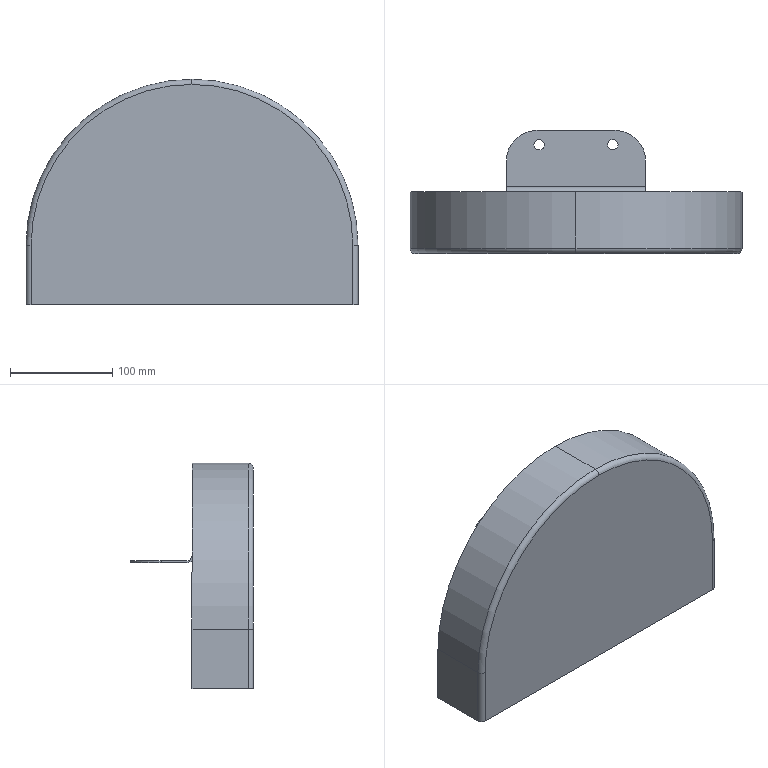Part | NX | features BREP 1 | 1 solid | 40 faces | box 324 x 120 x 220 mm | volume 283297 mm3 | cylinder 18 | plane 18 | torus 4 | commonest cylinder face diameters 10 x9 6 x2 60 x2 320 x2 324 x2 14 x1
STEP:
#1=CARTESIAN_POINT('',(193.612,71.603,383.));
#2=VERTEX_POINT('',#1);
#3=CARTESIAN_POINT('',(193.612,71.603,385.));
#4=VERTEX_POINT('',#3);
#5=CARTESIAN_POINT('',(193.612,71.603,326.345));
#6=DIRECTION('',(0.,0.,-1.));
#7=VECTOR('',#6,1000.);
#8=LINE('',#5,#7);
#9=EDGE_CURVE('',#2,#4,#8,.F.);
#10=ORIENTED_EDGE('',*,*,#9,.T.);
#11=CARTESIAN_POINT('',(202.388,76.397,385.));
#12=VERTEX_POINT('',#11);
#13=CARTESIAN_POINT('',(198.,74.,385.));
#14=DIRECTION('',(0.,0.,-1.));
#15=DIRECTION('',(1.,0.,0.));
#16=AXIS2_PLACEMENT_3D('',#13,#14,#15);
#17=CIRCLE('',#16,5.);
#18=EDGE_CURVE('',#12,#4,#17,.T.);
#19=ORIENTED_EDGE('',*,*,#18,.F.);
#20=CARTESIAN_POINT('',(202.388,76.397,383.));
#21=VERTEX_POINT('',#20);
#22=CARTESIAN_POINT('',(202.388,76.397,326.345));
#23=DIRECTION('',(0.,0.,-1.));
#24=VECTOR('',#23,1000.);
#25=LINE('',#22,#24);
#26=EDGE_CURVE('',#21,#12,#25,.F.);
#27=ORIENTED_EDGE('',*,*,#26,.F.);
#28=CARTESIAN_POINT('',(198.,74.,383.));
#29=DIRECTION('',(0.,0.,-1.));
#30=DIRECTION('',(1.,0.,0.));
#31=AXIS2_PLACEMENT_3D('',#28,#29,#30);
#32=CIRCLE('',#31,5.);
#33=EDGE_CURVE('',#21,#2,#32,.T.);
#34=ORIENTED_EDGE('',*,*,#33,.T.);
#35=EDGE_LOOP('',(#10,#19,#27,#34));
#36=FACE_BOUND('',#35,.T.);
#37=CARTESIAN_POINT('',(198.,74.,383.1));
#38=DIRECTION('',(0.,0.,1.));
#39=DIRECTION('',(-0.8776,-0.4794,0.));
#40=AXIS2_PLACEMENT_3D('',#37,#38,#39);
#41=CYLINDRICAL_SURFACE('',#40,5.);
#42=ADVANCED_FACE('',(#36),#41,.F.);
#43=ORIENTED_EDGE('',*,*,#26,.T.);
#44=CARTESIAN_POINT('',(198.,74.,385.));
#45=DIRECTION('',(0.,0.,-1.));
#46=DIRECTION('',(1.,0.,0.));
#47=AXIS2_PLACEMENT_3D('',#44,#45,#46);
#48=CIRCLE('',#47,5.);
#49=EDGE_CURVE('',#4,#12,#48,.T.);
#50=ORIENTED_EDGE('',*,*,#49,.F.);
#51=ORIENTED_EDGE('',*,*,#9,.F.);
#52=CARTESIAN_POINT('',(198.,74.,383.));
#53=DIRECTION('',(0.,0.,-1.));
#54=DIRECTION('',(1.,0.,0.));
#55=AXIS2_PLACEMENT_3D('',#52,#53,#54);
#56=CIRCLE('',#55,5.);
#57=EDGE_CURVE('',#2,#21,#56,.T.);
#58=ORIENTED_EDGE('',*,*,#57,.T.);
#59=EDGE_LOOP('',(#43,#50,#51,#58));
#60=FACE_BOUND('',#59,.T.);
#61=CARTESIAN_POINT('',(198.,74.,383.1));
#62=DIRECTION('',(0.,0.,1.));
#63=DIRECTION('',(-0.8776,-0.4794,0.));
#64=AXIS2_PLACEMENT_3D('',#61,#62,#63);
#65=CYLINDRICAL_SURFACE('',#64,5.);
#66=ADVANCED_FACE('',(#60),#65,.F.);
#67=CARTESIAN_POINT('',(240.,26.,393.));
#68=VERTEX_POINT('',#67);
#69=CARTESIAN_POINT('',(230.,26.,393.));
#70=VERTEX_POINT('',#69);
#71=CARTESIAN_POINT('',(235.,26.,393.));
#72=DIRECTION('',(-1.,0.,0.));
#73=VECTOR('',#72,1000.);
#74=LINE('',#71,#73);
#75=EDGE_CURVE('',#68,#70,#74,.T.);
#76=ORIENTED_EDGE('',*,*,#75,.T.);
#77=CARTESIAN_POINT('',(230.,28.,393.));
#78=VERTEX_POINT('',#77);
#79=CARTESIAN_POINT('',(230.,27.,393.));
#80=DIRECTION('',(0.,-1.,0.));
#81=VECTOR('',#80,1000.);
#82=LINE('',#79,#81);
#83=EDGE_CURVE('',#78,#70,#82,.T.);
#84=ORIENTED_EDGE('',*,*,#83,.F.);
#85=CARTESIAN_POINT('',(240.,28.,393.));
#86=VERTEX_POINT('',#85);
#87=CARTESIAN_POINT('',(235.,28.,393.));
#88=DIRECTION('',(1.,0.,0.));
#89=VECTOR('',#88,1000.);
#90=LINE('',#87,#89);
#91=EDGE_CURVE('',#78,#86,#90,.T.);
#92=ORIENTED_EDGE('',*,*,#91,.T.);
#93=CARTESIAN_POINT('',(240.,27.,393.));
#94=DIRECTION('',(0.,-1.,0.));
#95=VECTOR('',#94,1000.);
#96=LINE('',#93,#95);
#97=EDGE_CURVE('',#86,#68,#96,.T.);
#98=ORIENTED_EDGE('',*,*,#97,.T.);
#99=EDGE_LOOP('',(#76,#84,#92,#98));
#100=FACE_BOUND('',#99,.T.);
#101=CARTESIAN_POINT('',(94.,28.,393.));
#102=DIRECTION('',(0.,0.,1.));
#103=DIRECTION('',(1.,0.,0.));
#104=AXIS2_PLACEMENT_3D('',#101,#102,#103);
#105=PLANE('',#104);
#106=ADVANCED_FACE('',(#100),#105,.F.);
#107=CARTESIAN_POINT('',(94.,33.,385.));
#108=VERTEX_POINT('',#107);
#109=CARTESIAN_POINT('',(230.,33.,385.));
#110=VERTEX_POINT('',#109);
#111=CARTESIAN_POINT('',(162.,33.,385.));
#112=DIRECTION('',(1.,0.,0.));
#113=VECTOR('',#112,1000.);
#114=LINE('',#111,#113);
#115=EDGE_CURVE('',#108,#110,#114,.T.);
#116=ORIENTED_EDGE('',*,*,#115,.F.);
#117=CARTESIAN_POINT('',(94.,28.,390.));
#118=VERTEX_POINT('',#117);
#119=CARTESIAN_POINT('',(94.,33.,390.));
#120=DIRECTION('',(1.,0.,0.));
#121=DIRECTION('',(0.,0.,-1.));
#122=AXIS2_PLACEMENT_3D('',#119,#120,#121);
#123=CIRCLE('',#122,5.);
#124=EDGE_CURVE('',#118,#108,#123,.T.);
#125=ORIENTED_EDGE('',*,*,#124,.F.);
#126=CARTESIAN_POINT('',(230.,28.,390.));
#127=VERTEX_POINT('',#126);
#128=CARTESIAN_POINT('',(162.,28.,390.));
#129=DIRECTION('',(1.,0.,0.));
#130=VECTOR('',#129,1000.);
#131=LINE('',#128,#130);
#132=EDGE_CURVE('',#118,#127,#131,.T.);
#133=ORIENTED_EDGE('',*,*,#132,.T.);
#134=CARTESIAN_POINT('',(230.,33.,390.));
#135=DIRECTION('',(-1.,0.,0.));
#136=DIRECTION('',(0.,0.,-1.));
#137=AXIS2_PLACEMENT_3D('',#134,#135,#136);
#138=CIRCLE('',#137,5.);
#139=EDGE_CURVE('',#110,#127,#138,.T.);
#140=ORIENTED_EDGE('',*,*,#139,.F.);
#141=EDGE_LOOP('',(#116,#125,#133,#140));
#142=FACE_BOUND('',#141,.T.);
#143=CARTESIAN_POINT('',(162.,33.,390.));
#144=DIRECTION('',(1.,0.,0.));
#145=DIRECTION('',(0.,1.,0.));
#146=AXIS2_PLACEMENT_3D('',#143,#144,#145);
#147=CYLINDRICAL_SURFACE('',#146,5.);
#148=ADVANCED_FACE('',(#142),#147,.F.);
#149=CARTESIAN_POINT('',(94.,26.,393.));
#150=VERTEX_POINT('',#149);
#151=CARTESIAN_POINT('',(84.,26.,393.));
#152=VERTEX_POINT('',#151);
#153=CARTESIAN_POINT('',(89.,26.,393.));
#154=DIRECTION('',(-1.,0.,0.));
#155=VECTOR('',#154,1000.);
#156=LINE('',#153,#155);
#157=EDGE_CURVE('',#150,#152,#156,.T.);
#158=ORIENTED_EDGE('',*,*,#157,.T.);
#159=CARTESIAN_POINT('',(84.,28.,393.));
#160=VERTEX_POINT('',#159);
#161=CARTESIAN_POINT('',(84.,27.,393.));
#162=DIRECTION('',(0.,-1.,0.));
#163=VECTOR('',#162,1000.);
#164=LINE('',#161,#163);
#165=EDGE_CURVE('',#160,#152,#164,.T.);
#166=ORIENTED_EDGE('',*,*,#165,.F.);
#167=CARTESIAN_POINT('',(94.,28.,393.));
#168=VERTEX_POINT('',#167);
#169=CARTESIAN_POINT('',(89.,28.,393.));
#170=DIRECTION('',(1.,0.,0.));
#171=VECTOR('',#170,1000.);
#172=LINE('',#169,#171);
#173=EDGE_CURVE('',#160,#168,#172,.T.);
#174=ORIENTED_EDGE('',*,*,#173,.T.);
#175=CARTESIAN_POINT('',(94.,27.,393.));
#176=DIRECTION('',(0.,-1.,0.));
#177=VECTOR('',#176,1000.);
#178=LINE('',#175,#177);
#179=EDGE_CURVE('',#168,#150,#178,.T.);
#180=ORIENTED_EDGE('',*,*,#179,.T.);
#181=EDGE_LOOP('',(#158,#166,#174,#180));
#182=FACE_BOUND('',#181,.T.);
#183=CARTESIAN_POINT('',(94.,28.,393.));
#184=DIRECTION('',(0.,0.,1.));
#185=DIRECTION('',(1.,0.,0.));
#186=AXIS2_PLACEMENT_3D('',#183,#184,#185);
#187=PLANE('',#186);
#188=ADVANCED_FACE('',(#182),#187,.F.);
#189=CARTESIAN_POINT('',(230.,33.,383.));
#190=VERTEX_POINT('',#189);
#191=CARTESIAN_POINT('',(230.,26.,390.));
#192=VERTEX_POINT('',#191);
#193=CARTESIAN_POINT('',(230.,33.,390.));
#194=DIRECTION('',(-1.,0.,0.));
#195=DIRECTION('',(0.,0.,-1.));
#196=AXIS2_PLACEMENT_3D('',#193,#194,#195);
#197=CIRCLE('',#196,7.);
#198=EDGE_CURVE('',#190,#192,#197,.T.);
#199=ORIENTED_EDGE('',*,*,#198,.T.);
#200=CARTESIAN_POINT('',(94.,26.,390.));
#201=VERTEX_POINT('',#200);
#202=CARTESIAN_POINT('',(162.,26.,390.));
#203=DIRECTION('',(1.,0.,0.));
#204=VECTOR('',#203,1000.);
#205=LINE('',#202,#204);
#206=EDGE_CURVE('',#201,#192,#205,.T.);
#207=ORIENTED_EDGE('',*,*,#206,.F.);
#208=CARTESIAN_POINT('',(94.,33.,383.));
#209=VERTEX_POINT('',#208);
#210=CARTESIAN_POINT('',(94.,33.,390.));
#211=DIRECTION('',(1.,0.,0.));
#212=DIRECTION('',(0.,0.,-1.));
#213=AXIS2_PLACEMENT_3D('',#210,#211,#212);
#214=CIRCLE('',#213,7.);
#215=EDGE_CURVE('',#201,#209,#214,.T.);
#216=ORIENTED_EDGE('',*,*,#215,.T.);
#217=CARTESIAN_POINT('',(162.,33.,383.));
#218=DIRECTION('',(1.,0.,0.));
#219=VECTOR('',#218,1000.);
#220=LINE('',#217,#219);
#221=EDGE_CURVE('',#209,#190,#220,.T.);
#222=ORIENTED_EDGE('',*,*,#221,.T.);
#223=EDGE_LOOP('',(#199,#207,#216,#222));
#224=FACE_BOUND('',#223,.T.);
#225=CARTESIAN_POINT('',(162.,33.,390.));
#226=DIRECTION('',(1.,0.,0.));
#227=DIRECTION('',(0.,1.,0.));
#228=AXIS2_PLACEMENT_3D('',#225,#226,#227);
#229=CYLINDRICAL_SURFACE('',#228,7.);
#230=ADVANCED_FACE('',(#224),#229,.T.);
#231=CARTESIAN_POINT('',(121.612,71.603,383.));
#232=VERTEX_POINT('',#231);
#233=CARTESIAN_POINT('',(121.612,71.603,385.));
#234=VERTEX_POINT('',#233);
#235=CARTESIAN_POINT('',(121.612,71.603,326.345));
#236=DIRECTION('',(0.,0.,-1.));
#237=VECTOR('',#236,1000.);
#238=LINE('',#235,#237);
#239=EDGE_CURVE('',#232,#234,#238,.F.);
#240=ORIENTED_EDGE('',*,*,#239,.T.);
#241=CARTESIAN_POINT('',(130.388,76.397,385.));
#242=VERTEX_POINT('',#241);
#243=CARTESIAN_POINT('',(126.,74.,385.));
#244=DIRECTION('',(0.,0.,-1.));
#245=DIRECTION('',(1.,0.,0.));
#246=AXIS2_PLACEMENT_3D('',#243,#244,#245);
#247=CIRCLE('',#246,5.);
#248=EDGE_CURVE('',#242,#234,#247,.T.);
#249=ORIENTED_EDGE('',*,*,#248,.F.);
#250=CARTESIAN_POINT('',(130.388,76.397,383.));
#251=VERTEX_POINT('',#250);
#252=CARTESIAN_POINT('',(130.388,76.397,326.345));
#253=DIRECTION('',(0.,0.,-1.));
#254=VECTOR('',#253,1000.);
#255=LINE('',#252,#254);
#256=EDGE_CURVE('',#251,#242,#255,.F.);
#257=ORIENTED_EDGE('',*,*,#256,.F.);
#258=CARTESIAN_POINT('',(126.,74.,383.));
#259=DIRECTION('',(0.,0.,-1.));
#260=DIRECTION('',(1.,0.,0.));
#261=AXIS2_PLACEMENT_3D('',#258,#259,#260);
#262=CIRCLE('',#261,5.);
#263=EDGE_CURVE('',#251,#232,#262,.T.);
#264=ORIENTED_EDGE('',*,*,#263,.T.);
#265=EDGE_LOOP('',(#240,#249,#257,#264));
#266=FACE_BOUND('',#265,.T.);
#267=CARTESIAN_POINT('',(126.,74.,383.1));
#268=DIRECTION('',(0.,0.,1.));
#269=DIRECTION('',(-0.8776,-0.4794,0.));
#270=AXIS2_PLACEMENT_3D('',#267,#268,#269);
#271=CYLINDRICAL_SURFACE('',#270,5.);
#272=ADVANCED_FACE('',(#266),#271,.F.);
#273=ORIENTED_EDGE('',*,*,#256,.T.);
#274=CARTESIAN_POINT('',(126.,74.,385.));
#275=DIRECTION('',(0.,0.,-1.));
#276=DIRECTION('',(1.,0.,0.));
#277=AXIS2_PLACEMENT_3D('',#274,#275,#276);
#278=CIRCLE('',#277,5.);
#279=EDGE_CURVE('',#234,#242,#278,.T.);
#280=ORIENTED_EDGE('',*,*,#279,.F.);
#281=ORIENTED_EDGE('',*,*,#239,.F.);
#282=CARTESIAN_POINT('',(126.,74.,383.));
#283=DIRECTION('',(0.,0.,-1.));
#284=DIRECTION('',(1.,0.,0.));
#285=AXIS2_PLACEMENT_3D('',#282,#283,#284);
#286=CIRCLE('',#285,5.);
#287=EDGE_CURVE('',#232,#251,#286,.T.);
#288=ORIENTED_EDGE('',*,*,#287,.T.);
#289=EDGE_LOOP('',(#273,#280,#281,#288));
#290=FACE_BOUND('',#289,.T.);
#291=CARTESIAN_POINT('',(126.,74.,383.1));
#292=DIRECTION('',(0.,0.,1.));
#293=DIRECTION('',(-0.8776,-0.4794,0.));
#294=AXIS2_PLACEMENT_3D('',#291,#292,#293);
#295=CYLINDRICAL_SURFACE('',#294,5.);
#296=ADVANCED_FACE('',(#290),#295,.F.);
#297=CARTESIAN_POINT('',(94.,58.,383.));
#298=VERTEX_POINT('',#297);
#299=CARTESIAN_POINT('',(94.,58.,385.));
#300=VERTEX_POINT('',#299);
#301=CARTESIAN_POINT('',(94.,58.,384.));
#302=DIRECTION('',(0.,0.,1.));
#303=VECTOR('',#302,1000.);
#304=LINE('',#301,#303);
#305=EDGE_CURVE('',#298,#300,#304,.T.);
#306=ORIENTED_EDGE('',*,*,#305,.F.);
#307=CARTESIAN_POINT('',(94.,45.5,383.));
#308=DIRECTION('',(0.,-1.,0.));
#309=VECTOR('',#308,1000.);
#310=LINE('',#307,#309);
#311=EDGE_CURVE('',#298,#209,#310,.T.);
#312=ORIENTED_EDGE('',*,*,#311,.T.);
#313=ORIENTED_EDGE('',*,*,#215,.F.);
#314=CARTESIAN_POINT('',(94.,26.,391.5));
#315=DIRECTION('',(0.,0.,-1.));
#316=VECTOR('',#315,1000.);
#317=LINE('',#314,#316);
#318=EDGE_CURVE('',#150,#201,#317,.T.);
#319=ORIENTED_EDGE('',*,*,#318,.F.);
#320=ORIENTED_EDGE('',*,*,#179,.F.);
#321=CARTESIAN_POINT('',(94.,28.,391.5));
#322=DIRECTION('',(0.,0.,-1.));
#323=VECTOR('',#322,1000.);
#324=LINE('',#321,#323);
#325=EDGE_CURVE('',#168,#118,#324,.T.);
#326=ORIENTED_EDGE('',*,*,#325,.T.);
#327=ORIENTED_EDGE('',*,*,#124,.T.);
#328=CARTESIAN_POINT('',(94.,45.5,385.));
#329=DIRECTION('',(0.,1.,0.));
#330=VECTOR('',#329,1000.);
#331=LINE('',#328,#330);
#332=EDGE_CURVE('',#108,#300,#331,.T.);
#333=ORIENTED_EDGE('',*,*,#332,.T.);
#334=EDGE_LOOP('',(#306,#312,#313,#319,#320,#326,#327,#333));
#335=FACE_BOUND('',#334,.T.);
#336=CARTESIAN_POINT('',(94.,28.,383.));
#337=DIRECTION('',(1.,0.,0.));
#338=DIRECTION('',(0.,-1.,0.));
#339=AXIS2_PLACEMENT_3D('',#336,#337,#338);
#340=PLANE('',#339);
#341=ADVANCED_FACE('',(#335),#340,.F.);
#342=CARTESIAN_POINT('',(124.,88.,385.));
#343=VERTEX_POINT('',#342);
#344=CARTESIAN_POINT('',(124.,58.,385.));
#345=DIRECTION('',(0.,0.,-1.));
#346=DIRECTION('',(1.,0.,0.));
#347=AXIS2_PLACEMENT_3D('',#344,#345,#346);
#348=CIRCLE('',#347,30.);
#349=EDGE_CURVE('',#300,#343,#348,.T.);
#350=ORIENTED_EDGE('',*,*,#349,.T.);
#351=CARTESIAN_POINT('',(124.,88.,383.));
#352=VERTEX_POINT('',#351);
#353=CARTESIAN_POINT('',(124.,88.,388.));
#354=DIRECTION('',(0.,0.,1.));
#355=VECTOR('',#354,1000.);
#356=LINE('',#353,#355);
#357=EDGE_CURVE('',#352,#343,#356,.T.);
#358=ORIENTED_EDGE('',*,*,#357,.F.);
#359=CARTESIAN_POINT('',(124.,58.,383.));
#360=DIRECTION('',(0.,0.,1.));
#361=DIRECTION('',(1.,0.,0.));
#362=AXIS2_PLACEMENT_3D('',#359,#360,#361);
#363=CIRCLE('',#362,30.);
#364=EDGE_CURVE('',#352,#298,#363,.T.);
#365=ORIENTED_EDGE('',*,*,#364,.T.);
#366=ORIENTED_EDGE('',*,*,#305,.T.);
#367=EDGE_LOOP('',(#350,#358,#365,#366));
#368=FACE_BOUND('',#367,.T.);
#369=CARTESIAN_POINT('',(124.,58.,388.));
#370=DIRECTION('',(0.,0.,1.));
#371=DIRECTION('',(0.,-1.,0.));
#372=AXIS2_PLACEMENT_3D('',#369,#370,#371);
#373=CYLINDRICAL_SURFACE('',#372,30.);
#374=ADVANCED_FACE('',(#368),#373,.T.);
#375=CARTESIAN_POINT('',(230.,58.,383.));
#376=VERTEX_POINT('',#375);
#377=CARTESIAN_POINT('',(230.,58.,385.));
#378=VERTEX_POINT('',#377);
#379=CARTESIAN_POINT('',(230.,58.,384.));
#380=DIRECTION('',(0.,0.,1.));
#381=VECTOR('',#380,1000.);
#382=LINE('',#379,#381);
#383=EDGE_CURVE('',#376,#378,#382,.T.);
#384=ORIENTED_EDGE('',*,*,#383,.T.);
#385=CARTESIAN_POINT('',(230.,45.5,385.));
#386=DIRECTION('',(0.,-1.,0.));
#387=VECTOR('',#386,1000.);
#388=LINE('',#385,#387);
#389=EDGE_CURVE('',#378,#110,#388,.T.);
#390=ORIENTED_EDGE('',*,*,#389,.T.);
#391=ORIENTED_EDGE('',*,*,#139,.T.);
#392=CARTESIAN_POINT('',(230.,28.,391.5));
#393=DIRECTION('',(0.,0.,1.));
#394=VECTOR('',#393,1000.);
#395=LINE('',#392,#394);
#396=EDGE_CURVE('',#127,#78,#395,.T.);
#397=ORIENTED_EDGE('',*,*,#396,.T.);
#398=ORIENTED_EDGE('',*,*,#83,.T.);
#399=CARTESIAN_POINT('',(230.,26.,391.5));
#400=DIRECTION('',(0.,0.,-1.));
#401=VECTOR('',#400,1000.);
#402=LINE('',#399,#401);
#403=EDGE_CURVE('',#70,#192,#402,.T.);
#404=ORIENTED_EDGE('',*,*,#403,.T.);
#405=ORIENTED_EDGE('',*,*,#198,.F.);
#406=CARTESIAN_POINT('',(230.,45.5,383.));
#407=DIRECTION('',(0.,-1.,0.));
#408=VECTOR('',#407,1000.);
#409=LINE('',#406,#408);
#410=EDGE_CURVE('',#376,#190,#409,.T.);
#411=ORIENTED_EDGE('',*,*,#410,.F.);
#412=EDGE_LOOP('',(#384,#390,#391,#397,#398,#404,#405,#411));
#413=FACE_BOUND('',#412,.T.);
#414=CARTESIAN_POINT('',(230.,88.,383.));
#415=DIRECTION('',(-1.,0.,0.));
#416=DIRECTION('',(0.,1.,0.));
#417=AXIS2_PLACEMENT_3D('',#414,#415,#416);
#418=PLANE('',#417);
#419=ADVANCED_FACE('',(#413),#418,.F.);
#420=CARTESIAN_POINT('',(200.,88.,383.));
#421=VERTEX_POINT('',#420);
#422=CARTESIAN_POINT('',(162.,88.,383.));
#423=DIRECTION('',(1.,0.,0.));
#424=VECTOR('',#423,1000.);
#425=LINE('',#422,#424);
#426=EDGE_CURVE('',#352,#421,#425,.T.);
#427=ORIENTED_EDGE('',*,*,#426,.F.);
#428=ORIENTED_EDGE('',*,*,#357,.T.);
#429=CARTESIAN_POINT('',(200.,88.,385.));
#430=VERTEX_POINT('',#429);
#431=CARTESIAN_POINT('',(162.,88.,385.));
#432=DIRECTION('',(1.,0.,0.));
#433=VECTOR('',#432,1000.);
#434=LINE('',#431,#433);
#435=EDGE_CURVE('',#343,#430,#434,.T.);
#436=ORIENTED_EDGE('',*,*,#435,.T.);
#437=CARTESIAN_POINT('',(200.,88.,384.));
#438=DIRECTION('',(0.,0.,1.));
#439=VECTOR('',#438,1000.);
#440=LINE('',#437,#439);
#441=EDGE_CURVE('',#421,#430,#440,.T.);
#442=ORIENTED_EDGE('',*,*,#441,.F.);
#443=EDGE_LOOP('',(#427,#428,#436,#442));
#444=FACE_BOUND('',#443,.T.);
#445=CARTESIAN_POINT('',(230.,88.,383.));
#446=DIRECTION('',(0.,1.,0.));
#447=DIRECTION('',(1.,0.,0.));
#448=AXIS2_PLACEMENT_3D('',#445,#446,#447);
#449=PLANE('',#448);
#450=ADVANCED_FACE('',(#444),#449,.T.);
#451=CARTESIAN_POINT('',(200.,58.,385.));
#452=DIRECTION('',(0.,0.,-1.));
#453=DIRECTION('',(-1.,0.,0.));
#454=AXIS2_PLACEMENT_3D('',#451,#452,#453);
#455=CIRCLE('',#454,30.);
#456=EDGE_CURVE('',#430,#378,#455,.T.);
#457=ORIENTED_EDGE('',*,*,#456,.F.);
#458=ORIENTED_EDGE('',*,*,#435,.F.);
#459=ORIENTED_EDGE('',*,*,#349,.F.);
#460=ORIENTED_EDGE('',*,*,#332,.F.);
#461=ORIENTED_EDGE('',*,*,#115,.T.);
#462=ORIENTED_EDGE('',*,*,#389,.F.);
#463=EDGE_LOOP('',(#457,#458,#459,#460,#461,#462));
#464=FACE_BOUND('',#463,.T.);
#465=ORIENTED_EDGE('',*,*,#279,.T.);
#466=ORIENTED_EDGE('',*,*,#248,.T.);
#467=EDGE_LOOP('',(#465,#466));
#468=FACE_BOUND('',#467,.T.);
#469=ORIENTED_EDGE('',*,*,#18,.T.);
#470=ORIENTED_EDGE('',*,*,#49,.T.);
#471=EDGE_LOOP('',(#469,#470));
#472=FACE_BOUND('',#471,.T.);
#473=CARTESIAN_POINT('',(0.,0.,385.));
#474=DIRECTION('',(0.,0.,-1.));
#475=DIRECTION('',(-1.,0.,0.));
#476=AXIS2_PLACEMENT_3D('',#473,#474,#475);
#477=PLANE('',#476);
#478=ADVANCED_FACE('',(#464,#468,#472),#477,.F.);
#479=ORIENTED_EDGE('',*,*,#410,.T.);
#480=ORIENTED_EDGE('',*,*,#221,.F.);
#481=ORIENTED_EDGE('',*,*,#311,.F.);
#482=ORIENTED_EDGE('',*,*,#364,.F.);
#483=ORIENTED_EDGE('',*,*,#426,.T.);
#484=CARTESIAN_POINT('',(200.,58.,383.));
#485=DIRECTION('',(0.,0.,1.));
#486=DIRECTION('',(-1.,0.,0.));
#487=AXIS2_PLACEMENT_3D('',#484,#485,#486);
#488=CIRCLE('',#487,30.);
#489=EDGE_CURVE('',#376,#421,#488,.T.);
#490=ORIENTED_EDGE('',*,*,#489,.F.);
#491=EDGE_LOOP('',(#479,#480,#481,#482,#483,#490));
#492=FACE_BOUND('',#491,.T.);
#493=ORIENTED_EDGE('',*,*,#263,.F.);
#494=ORIENTED_EDGE('',*,*,#287,.F.);
#495=EDGE_LOOP('',(#493,#494));
#496=FACE_BOUND('',#495,.T.);
#497=ORIENTED_EDGE('',*,*,#57,.F.);
#498=ORIENTED_EDGE('',*,*,#33,.F.);
#499=EDGE_LOOP('',(#497,#498));
#500=FACE_BOUND('',#499,.T.);
#501=CARTESIAN_POINT('',(0.,0.,383.));
#502=DIRECTION('',(0.,0.,-1.));
#503=DIRECTION('',(-1.,0.,0.));
#504=AXIS2_PLACEMENT_3D('',#501,#502,#503);
#505=PLANE('',#504);
#506=ADVANCED_FACE('',(#492,#496,#500),#505,.T.);
#507=ORIENTED_EDGE('',*,*,#456,.T.);
#508=ORIENTED_EDGE('',*,*,#383,.F.);
#509=ORIENTED_EDGE('',*,*,#489,.T.);
#510=ORIENTED_EDGE('',*,*,#441,.T.);
#511=EDGE_LOOP('',(#507,#508,#509,#510));
#512=FACE_BOUND('',#511,.T.);
#513=CARTESIAN_POINT('',(200.,58.,388.));
#514=DIRECTION('',(0.,0.,1.));
#515=DIRECTION('',(-1.,0.,0.));
#516=AXIS2_PLACEMENT_3D('',#513,#514,#515);
#517=CYLINDRICAL_SURFACE('',#516,30.);
#518=ADVANCED_FACE('',(#512),#517,.T.);
#519=CARTESIAN_POINT('',(240.,28.,265.));
#520=VERTEX_POINT('',#519);
#521=CARTESIAN_POINT('',(240.,26.,265.));
#522=VERTEX_POINT('',#521);
#523=CARTESIAN_POINT('',(240.,27.,265.));
#524=DIRECTION('',(0.,-1.,0.));
#525=VECTOR('',#524,1000.);
#526=LINE('',#523,#525);
#527=EDGE_CURVE('',#520,#522,#526,.T.);
#528=ORIENTED_EDGE('',*,*,#527,.T.);
#529=CARTESIAN_POINT('',(240.,26.,329.));
#530=DIRECTION('',(0.,0.,1.));
#531=VECTOR('',#530,1000.);
#532=LINE('',#529,#531);
#533=EDGE_CURVE('',#522,#68,#532,.T.);
#534=ORIENTED_EDGE('',*,*,#533,.T.);
#535=ORIENTED_EDGE('',*,*,#97,.F.);
#536=CARTESIAN_POINT('',(240.,28.,329.));
#537=DIRECTION('',(0.,0.,-1.));
#538=VECTOR('',#537,1000.);
#539=LINE('',#536,#538);
#540=EDGE_CURVE('',#86,#520,#539,.T.);
#541=ORIENTED_EDGE('',*,*,#540,.T.);
#542=EDGE_LOOP('',(#528,#534,#535,#541));
#543=FACE_BOUND('',#542,.T.);
#544=CARTESIAN_POINT('',(240.,28.,217.524));
#545=DIRECTION('',(1.,0.,0.));
#546=DIRECTION('',(0.,0.,-1.));
#547=AXIS2_PLACEMENT_3D('',#544,#545,#546);
#548=PLANE('',#547);
#549=ADVANCED_FACE('',(#543),#548,.F.);
#550=CARTESIAN_POINT('',(245.,26.,260.));
#551=VERTEX_POINT('',#550);
#552=CARTESIAN_POINT('',(245.,26.,265.));
#553=DIRECTION('',(0.,1.,0.));
#554=DIRECTION('',(1.,0.,0.));
#555=AXIS2_PLACEMENT_3D('',#552,#553,#554);
#556=CIRCLE('',#555,5.);
#557=EDGE_CURVE('',#551,#522,#556,.T.);
#558=ORIENTED_EDGE('',*,*,#557,.T.);
#559=ORIENTED_EDGE('',*,*,#527,.F.);
#560=CARTESIAN_POINT('',(245.,28.,260.));
#561=VERTEX_POINT('',#560);
#562=CARTESIAN_POINT('',(245.,28.,265.));
#563=DIRECTION('',(0.,-1.,0.));
#564=DIRECTION('',(1.,0.,0.));
#565=AXIS2_PLACEMENT_3D('',#562,#563,#564);
#566=CIRCLE('',#565,5.);
#567=EDGE_CURVE('',#520,#561,#566,.T.);
#568=ORIENTED_EDGE('',*,*,#567,.T.);
#569=CARTESIAN_POINT('',(245.,-2.,260.));
#570=DIRECTION('',(0.,-1.,0.));
#571=VECTOR('',#570,1000.);
#572=LINE('',#569,#571);
#573=EDGE_CURVE('',#561,#551,#572,.T.);
#574=ORIENTED_EDGE('',*,*,#573,.T.);
#575=EDGE_LOOP('',(#558,#559,#568,#574));
#576=FACE_BOUND('',#575,.T.);
#577=CARTESIAN_POINT('',(245.,-2.,265.));
#578=DIRECTION('',(0.,-1.,0.));
#579=DIRECTION('',(1.,0.,0.));
#580=AXIS2_PLACEMENT_3D('',#577,#578,#579);
#581=CYLINDRICAL_SURFACE('',#580,5.);
#582=ADVANCED_FACE('',(#576),#581,.T.);
#583=CARTESIAN_POINT('',(84.,28.,265.));
#584=VERTEX_POINT('',#583);
#585=CARTESIAN_POINT('',(84.,26.,265.));
#586=VERTEX_POINT('',#585);
#587=CARTESIAN_POINT('',(84.,27.,265.));
#588=DIRECTION('',(0.,-1.,0.));
#589=VECTOR('',#588,1000.);
#590=LINE('',#587,#589);
#591=EDGE_CURVE('',#584,#586,#590,.T.);
#592=ORIENTED_EDGE('',*,*,#591,.F.);
#593=CARTESIAN_POINT('',(84.,28.,329.));
#594=DIRECTION('',(0.,0.,1.));
#595=VECTOR('',#594,1000.);
#596=LINE('',#593,#595);
#597=EDGE_CURVE('',#584,#160,#596,.T.);
#598=ORIENTED_EDGE('',*,*,#597,.T.);
#599=ORIENTED_EDGE('',*,*,#165,.T.);
#600=CARTESIAN_POINT('',(84.,26.,329.));
#601=DIRECTION('',(0.,0.,1.));
#602=VECTOR('',#601,1000.);
#603=LINE('',#600,#602);
#604=EDGE_CURVE('',#586,#152,#603,.T.);
#605=ORIENTED_EDGE('',*,*,#604,.F.);
#606=EDGE_LOOP('',(#592,#598,#599,#605));
#607=FACE_BOUND('',#606,.T.);
#608=CARTESIAN_POINT('',(84.,28.,393.));
#609=DIRECTION('',(-1.,0.,0.));
#610=DIRECTION('',(0.,0.,1.));
#611=AXIS2_PLACEMENT_3D('',#608,#609,#610);
#612=PLANE('',#611);
#613=ADVANCED_FACE('',(#607),#612,.F.);
#614=ORIENTED_EDGE('',*,*,#604,.T.);
#615=ORIENTED_EDGE('',*,*,#157,.F.);
#616=ORIENTED_EDGE('',*,*,#318,.T.);
#617=ORIENTED_EDGE('',*,*,#206,.T.);
#618=ORIENTED_EDGE('',*,*,#403,.F.);
#619=ORIENTED_EDGE('',*,*,#75,.F.);
#620=ORIENTED_EDGE('',*,*,#533,.F.);
#621=ORIENTED_EDGE('',*,*,#557,.F.);
#622=CARTESIAN_POINT('',(322.,26.,260.));
#623=VERTEX_POINT('',#622);
#624=CARTESIAN_POINT('',(162.,26.,260.));
#625=DIRECTION('',(1.,0.,0.));
#626=VECTOR('',#625,1000.);
#627=LINE('',#624,#626);
#628=EDGE_CURVE('',#551,#623,#627,.T.);
#629=ORIENTED_EDGE('',*,*,#628,.T.);
#630=CARTESIAN_POINT('',(322.,26.,318.));
#631=VERTEX_POINT('',#630);
#632=CARTESIAN_POINT('',(322.,26.,369.));
#633=DIRECTION('',(0.,0.,1.));
#634=VECTOR('',#633,1000.);
#635=LINE('',#632,#634);
#636=EDGE_CURVE('',#623,#631,#635,.T.);
#637=ORIENTED_EDGE('',*,*,#636,.T.);
#638=CARTESIAN_POINT('',(162.,26.,478.));
#639=VERTEX_POINT('',#638);
#640=CARTESIAN_POINT('',(162.,26.,318.));
#641=DIRECTION('',(0.,-1.,0.));
#642=DIRECTION('',(0.,0.,-1.));
#643=AXIS2_PLACEMENT_3D('',#640,#641,#642);
#644=CIRCLE('',#643,160.);
#645=EDGE_CURVE('',#631,#639,#644,.T.);
#646=ORIENTED_EDGE('',*,*,#645,.T.);
#647=CARTESIAN_POINT('',(2.,26.,318.));
#648=VERTEX_POINT('',#647);
#649=CARTESIAN_POINT('',(162.,26.,318.));
#650=DIRECTION('',(0.,-1.,0.));
#651=DIRECTION('',(0.,0.,-1.));
#652=AXIS2_PLACEMENT_3D('',#649,#650,#651);
#653=CIRCLE('',#652,160.);
#654=EDGE_CURVE('',#639,#648,#653,.T.);
#655=ORIENTED_EDGE('',*,*,#654,.T.);
#656=CARTESIAN_POINT('',(2.,26.,260.));
#657=VERTEX_POINT('',#656);
#658=CARTESIAN_POINT('',(2.,26.,369.));
#659=DIRECTION('',(0.,0.,1.));
#660=VECTOR('',#659,1000.);
#661=LINE('',#658,#660);
#662=EDGE_CURVE('',#657,#648,#661,.T.);
#663=ORIENTED_EDGE('',*,*,#662,.F.);
#664=CARTESIAN_POINT('',(79.,26.,260.));
#665=VERTEX_POINT('',#664);
#666=CARTESIAN_POINT('',(162.,26.,260.));
#667=DIRECTION('',(1.,0.,0.));
#668=VECTOR('',#667,1000.);
#669=LINE('',#666,#668);
#670=EDGE_CURVE('',#657,#665,#669,.T.);
#671=ORIENTED_EDGE('',*,*,#670,.T.);
#672=CARTESIAN_POINT('',(79.,26.,265.));
#673=DIRECTION('',(0.,-1.,0.));
#674=DIRECTION('',(0.,0.,-1.));
#675=AXIS2_PLACEMENT_3D('',#672,#673,#674);
#676=CIRCLE('',#675,5.);
#677=EDGE_CURVE('',#586,#665,#676,.F.);
#678=ORIENTED_EDGE('',*,*,#677,.F.);
#679=EDGE_LOOP('',(#614,#615,#616,#617,#618,#619,#620,#621,#629,#637,#646,#655,#663,#671,#678));
#680=FACE_BOUND('',#679,.T.);
#681=CARTESIAN_POINT('',(94.,26.,383.));
#682=DIRECTION('',(0.,-1.,0.));
#683=DIRECTION('',(-1.,0.,0.));
#684=AXIS2_PLACEMENT_3D('',#681,#682,#683);
#685=PLANE('',#684);
#686=ADVANCED_FACE('',(#680),#685,.T.);
#687=CARTESIAN_POINT('',(79.,28.,260.));
#688=VERTEX_POINT('',#687);
#689=CARTESIAN_POINT('',(79.,28.,265.));
#690=DIRECTION('',(0.,-1.,0.));
#691=DIRECTION('',(1.,0.,0.));
#692=AXIS2_PLACEMENT_3D('',#689,#690,#691);
#693=CIRCLE('',#692,5.);
#694=EDGE_CURVE('',#688,#584,#693,.T.);
#695=ORIENTED_EDGE('',*,*,#694,.F.);
#696=CARTESIAN_POINT('',(0.,28.,260.));
#697=VERTEX_POINT('',#696);
#698=CARTESIAN_POINT('',(39.5,28.,260.));
#699=DIRECTION('',(1.,0.,0.));
#700=VECTOR('',#699,1000.);
#701=LINE('',#698,#700);
#702=EDGE_CURVE('',#697,#688,#701,.T.);
#703=ORIENTED_EDGE('',*,*,#702,.F.);
#704=CARTESIAN_POINT('',(0.,28.,318.));
#705=VERTEX_POINT('',#704);
#706=CARTESIAN_POINT('',(0.,28.,289.));
#707=DIRECTION('',(0.,0.,-1.));
#708=VECTOR('',#707,1000.);
#709=LINE('',#706,#708);
#710=EDGE_CURVE('',#705,#697,#709,.T.);
#711=ORIENTED_EDGE('',*,*,#710,.F.);
#712=CARTESIAN_POINT('',(162.,28.,480.));
#713=VERTEX_POINT('',#712);
#714=CARTESIAN_POINT('',(162.,28.,318.));
#715=DIRECTION('',(0.,-1.,0.));
#716=DIRECTION('',(1.,0.,0.));
#717=AXIS2_PLACEMENT_3D('',#714,#715,#716);
#718=CIRCLE('',#717,162.);
#719=EDGE_CURVE('',#713,#705,#718,.T.);
#720=ORIENTED_EDGE('',*,*,#719,.F.);
#721=CARTESIAN_POINT('',(324.,28.,318.));
#722=VERTEX_POINT('',#721);
#723=CARTESIAN_POINT('',(162.,28.,318.));
#724=DIRECTION('',(0.,-1.,0.));
#725=DIRECTION('',(1.,0.,0.));
#726=AXIS2_PLACEMENT_3D('',#723,#724,#725);
#727=CIRCLE('',#726,162.);
#728=EDGE_CURVE('',#722,#713,#727,.T.);
#729=ORIENTED_EDGE('',*,*,#728,.F.);
#730=CARTESIAN_POINT('',(324.,28.,260.));
#731=VERTEX_POINT('',#730);
#732=CARTESIAN_POINT('',(324.,28.,289.));
#733=DIRECTION('',(0.,0.,1.));
#734=VECTOR('',#733,1000.);
#735=LINE('',#732,#734);
#736=EDGE_CURVE('',#731,#722,#735,.T.);
#737=ORIENTED_EDGE('',*,*,#736,.F.);
#738=CARTESIAN_POINT('',(284.5,28.,260.));
#739=DIRECTION('',(1.,0.,0.));
#740=VECTOR('',#739,1000.);
#741=LINE('',#738,#740);
#742=EDGE_CURVE('',#561,#731,#741,.T.);
#743=ORIENTED_EDGE('',*,*,#742,.F.);
#744=ORIENTED_EDGE('',*,*,#567,.F.);
#745=ORIENTED_EDGE('',*,*,#540,.F.);
#746=ORIENTED_EDGE('',*,*,#91,.F.);
#747=ORIENTED_EDGE('',*,*,#396,.F.);
#748=ORIENTED_EDGE('',*,*,#132,.F.);
#749=ORIENTED_EDGE('',*,*,#325,.F.);
#750=ORIENTED_EDGE('',*,*,#173,.F.);
#751=ORIENTED_EDGE('',*,*,#597,.F.);
#752=EDGE_LOOP('',(#695,#703,#711,#720,#729,#737,#743,#744,#745,#746,#747,#748,#749,#750,#751));
#753=FACE_BOUND('',#752,.T.);
#754=CARTESIAN_POINT('',(94.,28.,383.));
#755=DIRECTION('',(0.,-1.,0.));
#756=DIRECTION('',(-1.,0.,0.));
#757=AXIS2_PLACEMENT_3D('',#754,#755,#756);
#758=PLANE('',#757);
#759=ADVANCED_FACE('',(#753),#758,.F.);
#760=ORIENTED_EDGE('',*,*,#677,.T.);
#761=CARTESIAN_POINT('',(79.,-2.,260.));
#762=DIRECTION('',(0.,-1.,0.));
#763=VECTOR('',#762,1000.);
#764=LINE('',#761,#763);
#765=EDGE_CURVE('',#688,#665,#764,.T.);
#766=ORIENTED_EDGE('',*,*,#765,.F.);
#767=ORIENTED_EDGE('',*,*,#694,.T.);
#768=ORIENTED_EDGE('',*,*,#591,.T.);
#769=EDGE_LOOP('',(#760,#766,#767,#768));
#770=FACE_BOUND('',#769,.T.);
#771=CARTESIAN_POINT('',(79.,-2.,265.));
#772=DIRECTION('',(0.,-1.,0.));
#773=DIRECTION('',(0.,0.,1.));
#774=AXIS2_PLACEMENT_3D('',#771,#772,#773);
#775=CYLINDRICAL_SURFACE('',#774,5.);
#776=ADVANCED_FACE('',(#770),#775,.T.);
#777=CARTESIAN_POINT('',(5.,-32.,260.));
#778=VERTEX_POINT('',#777);
#779=CARTESIAN_POINT('',(319.,-32.,260.));
#780=VERTEX_POINT('',#779);
#781=CARTESIAN_POINT('',(162.,-32.,260.));
#782=DIRECTION('',(1.,0.,0.));
#783=VECTOR('',#782,1000.);
#784=LINE('',#781,#783);
#785=EDGE_CURVE('',#778,#780,#784,.T.);
#786=ORIENTED_EDGE('',*,*,#785,.T.);
#787=CARTESIAN_POINT('',(319.,-32.,318.));
#788=VERTEX_POINT('',#787);
#789=CARTESIAN_POINT('',(319.,-32.,289.));
#790=DIRECTION('',(0.,0.,-1.));
#791=VECTOR('',#790,1000.);
#792=LINE('',#789,#791);
#793=EDGE_CURVE('',#788,#780,#792,.T.);
#794=ORIENTED_EDGE('',*,*,#793,.F.);
#795=CARTESIAN_POINT('',(162.,-32.,475.));
#796=VERTEX_POINT('',#795);
#797=CARTESIAN_POINT('',(162.,-32.,318.));
#798=DIRECTION('',(0.,1.,0.));
#799=DIRECTION('',(1.,0.,0.));
#800=AXIS2_PLACEMENT_3D('',#797,#798,#799);
#801=CIRCLE('',#800,157.);
#802=EDGE_CURVE('',#796,#788,#801,.T.);
#803=ORIENTED_EDGE('',*,*,#802,.F.);
#804=CARTESIAN_POINT('',(5.,-32.,318.));
#805=VERTEX_POINT('',#804);
#806=CARTESIAN_POINT('',(162.,-32.,318.));
#807=DIRECTION('',(0.,1.,0.));
#808=DIRECTION('',(1.,0.,0.));
#809=AXIS2_PLACEMENT_3D('',#806,#807,#808);
#810=CIRCLE('',#809,157.);
#811=EDGE_CURVE('',#805,#796,#810,.T.);
#812=ORIENTED_EDGE('',*,*,#811,.F.);
#813=CARTESIAN_POINT('',(5.,-32.,289.));
#814=DIRECTION('',(0.,0.,1.));
#815=VECTOR('',#814,1000.);
#816=LINE('',#813,#815);
#817=EDGE_CURVE('',#778,#805,#816,.T.);
#818=ORIENTED_EDGE('',*,*,#817,.F.);
#819=EDGE_LOOP('',(#786,#794,#803,#812,#818));
#820=FACE_BOUND('',#819,.T.);
#821=CARTESIAN_POINT('',(0.,-32.,0.));
#822=DIRECTION('',(0.,-1.,0.));
#823=DIRECTION('',(-1.,0.,0.));
#824=AXIS2_PLACEMENT_3D('',#821,#822,#823);
#825=PLANE('',#824);
#826=ADVANCED_FACE('',(#820),#825,.T.);
#827=CARTESIAN_POINT('',(0.,-27.,318.));
#828=VERTEX_POINT('',#827);
#829=CARTESIAN_POINT('',(0.,0.5,318.));
#830=DIRECTION('',(0.,-1.,0.));
#831=VECTOR('',#830,1000.);
#832=LINE('',#829,#831);
#833=EDGE_CURVE('',#705,#828,#832,.T.);
#834=ORIENTED_EDGE('',*,*,#833,.F.);
#835=ORIENTED_EDGE('',*,*,#710,.T.);
#836=CARTESIAN_POINT('',(0.,-27.,260.));
#837=VERTEX_POINT('',#836);
#838=CARTESIAN_POINT('',(0.,0.5,260.));
#839=DIRECTION('',(0.,-1.,0.));
#840=VECTOR('',#839,1000.);
#841=LINE('',#838,#840);
#842=EDGE_CURVE('',#697,#837,#841,.T.);
#843=ORIENTED_EDGE('',*,*,#842,.T.);
#844=CARTESIAN_POINT('',(0.,-27.,289.));
#845=DIRECTION('',(0.,0.,1.));
#846=VECTOR('',#845,1000.);
#847=LINE('',#844,#846);
#848=EDGE_CURVE('',#837,#828,#847,.T.);
#849=ORIENTED_EDGE('',*,*,#848,.T.);
#850=EDGE_LOOP('',(#834,#835,#843,#849));
#851=FACE_BOUND('',#850,.T.);
#852=CARTESIAN_POINT('',(0.,28.,480.));
#853=DIRECTION('',(-1.,0.,0.));
#854=DIRECTION('',(0.,0.,1.));
#855=AXIS2_PLACEMENT_3D('',#852,#853,#854);
#856=PLANE('',#855);
#857=ADVANCED_FACE('',(#851),#856,.T.);
#858=CARTESIAN_POINT('',(162.,-27.,480.));
#859=VERTEX_POINT('',#858);
#860=CARTESIAN_POINT('',(162.,-2.,480.));
#861=DIRECTION('',(0.,-1.,0.));
#862=VECTOR('',#861,1000.);
#863=LINE('',#860,#862);
#864=EDGE_CURVE('',#713,#859,#863,.T.);
#865=ORIENTED_EDGE('',*,*,#864,.F.);
#866=ORIENTED_EDGE('',*,*,#719,.T.);
#867=ORIENTED_EDGE('',*,*,#833,.T.);
#868=CARTESIAN_POINT('',(162.,-27.,318.));
#869=DIRECTION('',(0.,1.,0.));
#870=DIRECTION('',(1.,0.,0.));
#871=AXIS2_PLACEMENT_3D('',#868,#869,#870);
#872=CIRCLE('',#871,162.);
#873=EDGE_CURVE('',#828,#859,#872,.T.);
#874=ORIENTED_EDGE('',*,*,#873,.T.);
#875=EDGE_LOOP('',(#865,#866,#867,#874));
#876=FACE_BOUND('',#875,.T.);
#877=CARTESIAN_POINT('',(162.,-2.,318.));
#878=DIRECTION('',(0.,-1.,0.));
#879=DIRECTION('',(0.,0.,-1.));
#880=AXIS2_PLACEMENT_3D('',#877,#878,#879);
#881=CYLINDRICAL_SURFACE('',#880,162.);
#882=ADVANCED_FACE('',(#876),#881,.T.);
#883=CARTESIAN_POINT('',(324.,-27.,318.));
#884=VERTEX_POINT('',#883);
#885=CARTESIAN_POINT('',(324.,-2.,318.));
#886=DIRECTION('',(0.,-1.,0.));
#887=VECTOR('',#886,1000.);
#888=LINE('',#885,#887);
#889=EDGE_CURVE('',#722,#884,#888,.T.);
#890=ORIENTED_EDGE('',*,*,#889,.F.);
#891=ORIENTED_EDGE('',*,*,#728,.T.);
#892=ORIENTED_EDGE('',*,*,#864,.T.);
#893=CARTESIAN_POINT('',(162.,-27.,318.));
#894=DIRECTION('',(0.,1.,0.));
#895=DIRECTION('',(1.,0.,0.));
#896=AXIS2_PLACEMENT_3D('',#893,#894,#895);
#897=CIRCLE('',#896,162.);
#898=EDGE_CURVE('',#859,#884,#897,.T.);
#899=ORIENTED_EDGE('',*,*,#898,.T.);
#900=EDGE_LOOP('',(#890,#891,#892,#899));
#901=FACE_BOUND('',#900,.T.);
#902=CARTESIAN_POINT('',(162.,-2.,318.));
#903=DIRECTION('',(0.,-1.,0.));
#904=DIRECTION('',(-1.,0.,0.));
#905=AXIS2_PLACEMENT_3D('',#902,#903,#904);
#906=CYLINDRICAL_SURFACE('',#905,162.);
#907=ADVANCED_FACE('',(#901),#906,.T.);
#908=CARTESIAN_POINT('',(324.,-27.,260.));
#909=VERTEX_POINT('',#908);
#910=CARTESIAN_POINT('',(324.,0.5,260.));
#911=DIRECTION('',(0.,-1.,0.));
#912=VECTOR('',#911,1000.);
#913=LINE('',#910,#912);
#914=EDGE_CURVE('',#731,#909,#913,.T.);
#915=ORIENTED_EDGE('',*,*,#914,.F.);
#916=ORIENTED_EDGE('',*,*,#736,.T.);
#917=ORIENTED_EDGE('',*,*,#889,.T.);
#918=CARTESIAN_POINT('',(324.,-27.,289.));
#919=DIRECTION('',(0.,0.,-1.));
#920=VECTOR('',#919,1000.);
#921=LINE('',#918,#920);
#922=EDGE_CURVE('',#884,#909,#921,.T.);
#923=ORIENTED_EDGE('',*,*,#922,.T.);
#924=EDGE_LOOP('',(#915,#916,#917,#923));
#925=FACE_BOUND('',#924,.T.);
#926=CARTESIAN_POINT('',(324.,28.,260.));
#927=DIRECTION('',(1.,0.,0.));
#928=DIRECTION('',(0.,0.,-1.));
#929=AXIS2_PLACEMENT_3D('',#926,#927,#928);
#930=PLANE('',#929);
#931=ADVANCED_FACE('',(#925),#930,.T.);
#932=CARTESIAN_POINT('',(5.,-27.,318.));
#933=DIRECTION('',(0.000000001,0.,1.));
#934=DIRECTION('',(1.,0.,-0.000000001));
#935=AXIS2_PLACEMENT_3D('',#932,#933,#934);
#936=CIRCLE('',#935,5.);
#937=EDGE_CURVE('',#828,#805,#936,.T.);
#938=ORIENTED_EDGE('',*,*,#937,.T.);
#939=ORIENTED_EDGE('',*,*,#811,.T.);
#940=CARTESIAN_POINT('',(162.,-27.,475.));
#941=DIRECTION('',(1.,0.,0.));
#942=DIRECTION('',(0.,0.,-1.));
#943=AXIS2_PLACEMENT_3D('',#940,#941,#942);
#944=CIRCLE('',#943,5.);
#945=EDGE_CURVE('',#859,#796,#944,.T.);
#946=ORIENTED_EDGE('',*,*,#945,.F.);
#947=ORIENTED_EDGE('',*,*,#873,.F.);
#948=EDGE_LOOP('',(#938,#939,#946,#947));
#949=FACE_BOUND('',#948,.T.);
#950=CARTESIAN_POINT('',(162.,-27.,318.));
#951=DIRECTION('',(0.,-1.,0.));
#952=DIRECTION('',(-0.07368,0.,-0.9973));
#953=AXIS2_PLACEMENT_3D('',#950,#951,#952);
#954=TOROIDAL_SURFACE('',#953,157.,5.);
#955=ADVANCED_FACE('',(#949),#954,.T.);
#956=ORIENTED_EDGE('',*,*,#945,.T.);
#957=ORIENTED_EDGE('',*,*,#802,.T.);
#958=CARTESIAN_POINT('',(319.,-27.,318.));
#959=DIRECTION('',(0.,0.,-1.));
#960=DIRECTION('',(1.,0.,0.));
#961=AXIS2_PLACEMENT_3D('',#958,#959,#960);
#962=CIRCLE('',#961,5.);
#963=EDGE_CURVE('',#884,#788,#962,.T.);
#964=ORIENTED_EDGE('',*,*,#963,.F.);
#965=ORIENTED_EDGE('',*,*,#898,.F.);
#966=EDGE_LOOP('',(#956,#957,#964,#965));
#967=FACE_BOUND('',#966,.T.);
#968=CARTESIAN_POINT('',(162.,-27.,318.));
#969=DIRECTION('',(0.,-1.,0.));
#970=DIRECTION('',(-0.939,0.,0.3439));
#971=AXIS2_PLACEMENT_3D('',#968,#969,#970);
#972=TOROIDAL_SURFACE('',#971,157.,5.);
#973=ADVANCED_FACE('',(#967),#972,.T.);
#974=ORIENTED_EDGE('',*,*,#922,.F.);
#975=ORIENTED_EDGE('',*,*,#963,.T.);
#976=ORIENTED_EDGE('',*,*,#793,.T.);
#977=CARTESIAN_POINT('',(319.,-27.,260.));
#978=DIRECTION('',(0.,0.,1.));
#979=DIRECTION('',(1.,0.,0.));
#980=AXIS2_PLACEMENT_3D('',#977,#978,#979);
#981=CIRCLE('',#980,5.);
#982=EDGE_CURVE('',#780,#909,#981,.T.);
#983=ORIENTED_EDGE('',*,*,#982,.T.);
#984=EDGE_LOOP('',(#974,#975,#976,#983));
#985=FACE_BOUND('',#984,.T.);
#986=CARTESIAN_POINT('',(319.,-27.,370.));
#987=DIRECTION('',(0.,0.,1.));
#988=DIRECTION('',(0.,1.,0.));
#989=AXIS2_PLACEMENT_3D('',#986,#987,#988);
#990=CYLINDRICAL_SURFACE('',#989,5.);
#991=ADVANCED_FACE('',(#985),#990,.T.);
#992=ORIENTED_EDGE('',*,*,#817,.T.);
#993=ORIENTED_EDGE('',*,*,#937,.F.);
#994=ORIENTED_EDGE('',*,*,#848,.F.);
#995=CARTESIAN_POINT('',(5.,-27.,260.));
#996=DIRECTION('',(0.,0.,1.));
#997=DIRECTION('',(-1.,0.,0.));
#998=AXIS2_PLACEMENT_3D('',#995,#996,#997);
#999=CIRCLE('',#998,5.);
#1000=EDGE_CURVE('',#837,#778,#999,.T.);
#1001=ORIENTED_EDGE('',*,*,#1000,.T.);
#1002=EDGE_LOOP('',(#992,#993,#994,#1001));
#1003=FACE_BOUND('',#1002,.T.);
#1004=CARTESIAN_POINT('',(5.,-27.,370.));
#1005=DIRECTION('',(0.,0.,-1.));
#1006=DIRECTION('',(0.,1.,0.));
#1007=AXIS2_PLACEMENT_3D('',#1004,#1005,#1006);
#1008=CYLINDRICAL_SURFACE('',#1007,5.);
#1009=ADVANCED_FACE('',(#1003),#1008,.T.);
#1010=CARTESIAN_POINT('',(5.,-30.,260.));
#1011=VERTEX_POINT('',#1010);
#1012=CARTESIAN_POINT('',(319.,-30.,260.));
#1013=VERTEX_POINT('',#1012);
#1014=CARTESIAN_POINT('',(162.,-30.,260.));
#1015=DIRECTION('',(1.,0.,0.));
#1016=VECTOR('',#1015,1000.);
#1017=LINE('',#1014,#1016);
#1018=EDGE_CURVE('',#1011,#1013,#1017,.T.);
#1019=ORIENTED_EDGE('',*,*,#1018,.T.);
#1020=CARTESIAN_POINT('',(322.,-27.,260.));
#1021=VERTEX_POINT('',#1020);
#1022=CARTESIAN_POINT('',(319.,-27.,260.));
#1023=DIRECTION('',(0.,0.,1.));
#1024=DIRECTION('',(-1.,0.,0.));
#1025=AXIS2_PLACEMENT_3D('',#1022,#1023,#1024);
#1026=CIRCLE('',#1025,3.);
#1027=EDGE_CURVE('',#1013,#1021,#1026,.T.);
#1028=ORIENTED_EDGE('',*,*,#1027,.T.);
#1029=CARTESIAN_POINT('',(322.,-0.5,260.));
#1030=DIRECTION('',(0.,-1.,0.));
#1031=VECTOR('',#1030,1000.);
#1032=LINE('',#1029,#1031);
#1033=EDGE_CURVE('',#623,#1021,#1032,.T.);
#1034=ORIENTED_EDGE('',*,*,#1033,.F.);
#1035=ORIENTED_EDGE('',*,*,#628,.F.);
#1036=ORIENTED_EDGE('',*,*,#573,.F.);
#1037=ORIENTED_EDGE('',*,*,#742,.T.);
#1038=ORIENTED_EDGE('',*,*,#914,.T.);
#1039=ORIENTED_EDGE('',*,*,#982,.F.);
#1040=ORIENTED_EDGE('',*,*,#785,.F.);
#1041=ORIENTED_EDGE('',*,*,#1000,.F.);
#1042=ORIENTED_EDGE('',*,*,#842,.F.);
#1043=ORIENTED_EDGE('',*,*,#702,.T.);
#1044=ORIENTED_EDGE('',*,*,#765,.T.);
#1045=ORIENTED_EDGE('',*,*,#670,.F.);
#1046=CARTESIAN_POINT('',(2.,-27.,260.));
#1047=VERTEX_POINT('',#1046);
#1048=CARTESIAN_POINT('',(2.,-0.5,260.));
#1049=DIRECTION('',(0.,-1.,0.));
#1050=VECTOR('',#1049,1000.);
#1051=LINE('',#1048,#1050);
#1052=EDGE_CURVE('',#657,#1047,#1051,.T.);
#1053=ORIENTED_EDGE('',*,*,#1052,.T.);
#1054=CARTESIAN_POINT('',(5.,-27.,260.));
#1055=DIRECTION('',(0.,0.,1.));
#1056=DIRECTION('',(-1.,0.,0.));
#1057=AXIS2_PLACEMENT_3D('',#1054,#1055,#1056);
#1058=CIRCLE('',#1057,3.);
#1059=EDGE_CURVE('',#1047,#1011,#1058,.T.);
#1060=ORIENTED_EDGE('',*,*,#1059,.T.);
#1061=EDGE_LOOP('',(#1019,#1028,#1034,#1035,#1036,#1037,#1038,#1039,#1040,#1041,#1042,#1043,#1044,#1045,#1053,#1060));
#1062=FACE_BOUND('',#1061,.T.);
#1063=CARTESIAN_POINT('',(0.,28.,260.));
#1064=DIRECTION('',(0.,0.,-1.));
#1065=DIRECTION('',(-1.,0.,0.));
#1066=AXIS2_PLACEMENT_3D('',#1063,#1064,#1065);
#1067=PLANE('',#1066);
#1068=ADVANCED_FACE('',(#1062),#1067,.T.);
#1069=CARTESIAN_POINT('',(322.,-27.,318.));
#1070=VERTEX_POINT('',#1069);
#1071=CARTESIAN_POINT('',(322.,-27.,289.));
#1072=DIRECTION('',(0.,0.,-1.));
#1073=VECTOR('',#1072,1000.);
#1074=LINE('',#1071,#1073);
#1075=EDGE_CURVE('',#1070,#1021,#1074,.T.);
#1076=ORIENTED_EDGE('',*,*,#1075,.F.);
#1077=CARTESIAN_POINT('',(322.,-2.,318.));
#1078=DIRECTION('',(0.,-1.,0.));
#1079=VECTOR('',#1078,1000.);
#1080=LINE('',#1077,#1079);
#1081=EDGE_CURVE('',#631,#1070,#1080,.T.);
#1082=ORIENTED_EDGE('',*,*,#1081,.F.);
#1083=ORIENTED_EDGE('',*,*,#636,.F.);
#1084=ORIENTED_EDGE('',*,*,#1033,.T.);
#1085=EDGE_LOOP('',(#1076,#1082,#1083,#1084));
#1086=FACE_BOUND('',#1085,.T.);
#1087=CARTESIAN_POINT('',(322.,28.,260.));
#1088=DIRECTION('',(1.,0.,0.));
#1089=DIRECTION('',(0.,0.,-1.));
#1090=AXIS2_PLACEMENT_3D('',#1087,#1088,#1089);
#1091=PLANE('',#1090);
#1092=ADVANCED_FACE('',(#1086),#1091,.F.);
#1093=CARTESIAN_POINT('',(162.,-27.,478.));
#1094=VERTEX_POINT('',#1093);
#1095=CARTESIAN_POINT('',(162.,-27.,318.));
#1096=DIRECTION('',(0.,1.,0.));
#1097=DIRECTION('',(1.,0.,0.));
#1098=AXIS2_PLACEMENT_3D('',#1095,#1096,#1097);
#1099=CIRCLE('',#1098,160.);
#1100=EDGE_CURVE('',#1094,#1070,#1099,.T.);
#1101=ORIENTED_EDGE('',*,*,#1100,.F.);
#1102=CARTESIAN_POINT('',(162.,-2.,478.));
#1103=DIRECTION('',(0.,-1.,0.));
#1104=VECTOR('',#1103,1000.);
#1105=LINE('',#1102,#1104);
#1106=EDGE_CURVE('',#639,#1094,#1105,.T.);
#1107=ORIENTED_EDGE('',*,*,#1106,.F.);
#1108=ORIENTED_EDGE('',*,*,#645,.F.);
#1109=ORIENTED_EDGE('',*,*,#1081,.T.);
#1110=EDGE_LOOP('',(#1101,#1107,#1108,#1109));
#1111=FACE_BOUND('',#1110,.T.);
#1112=CARTESIAN_POINT('',(162.,-2.,318.));
#1113=DIRECTION('',(0.,-1.,0.));
#1114=DIRECTION('',(0.7071,0.,0.7071));
#1115=AXIS2_PLACEMENT_3D('',#1112,#1113,#1114);
#1116=CYLINDRICAL_SURFACE('',#1115,160.);
#1117=ADVANCED_FACE('',(#1111),#1116,.F.);
#1118=CARTESIAN_POINT('',(2.,-27.,318.));
#1119=VERTEX_POINT('',#1118);
#1120=CARTESIAN_POINT('',(162.,-27.,318.));
#1121=DIRECTION('',(0.,1.,0.));
#1122=DIRECTION('',(1.,0.,0.));
#1123=AXIS2_PLACEMENT_3D('',#1120,#1121,#1122);
#1124=CIRCLE('',#1123,160.);
#1125=EDGE_CURVE('',#1119,#1094,#1124,.T.);
#1126=ORIENTED_EDGE('',*,*,#1125,.F.);
#1127=CARTESIAN_POINT('',(2.,-2.,318.));
#1128=DIRECTION('',(0.,-1.,0.));
#1129=VECTOR('',#1128,1000.);
#1130=LINE('',#1127,#1129);
#1131=EDGE_CURVE('',#648,#1119,#1130,.T.);
#1132=ORIENTED_EDGE('',*,*,#1131,.F.);
#1133=ORIENTED_EDGE('',*,*,#654,.F.);
#1134=ORIENTED_EDGE('',*,*,#1106,.T.);
#1135=EDGE_LOOP('',(#1126,#1132,#1133,#1134));
#1136=FACE_BOUND('',#1135,.T.);
#1137=CARTESIAN_POINT('',(162.,-2.,318.));
#1138=DIRECTION('',(0.,-1.,0.));
#1139=DIRECTION('',(-0.7071,0.,0.7071));
#1140=AXIS2_PLACEMENT_3D('',#1137,#1138,#1139);
#1141=CYLINDRICAL_SURFACE('',#1140,160.);
#1142=ADVANCED_FACE('',(#1136),#1141,.F.);
#1143=CARTESIAN_POINT('',(5.,-30.,318.));
#1144=VERTEX_POINT('',#1143);
#1145=CARTESIAN_POINT('',(5.,-30.,369.));
#1146=DIRECTION('',(0.,0.,1.));
#1147=VECTOR('',#1146,1000.);
#1148=LINE('',#1145,#1147);
#1149=EDGE_CURVE('',#1011,#1144,#1148,.T.);
#1150=ORIENTED_EDGE('',*,*,#1149,.T.);
#1151=CARTESIAN_POINT('',(162.,-30.,475.));
#1152=VERTEX_POINT('',#1151);
#1153=CARTESIAN_POINT('',(5.,-30.,318.));
#1154=CARTESIAN_POINT('',(5.,-30.,342.662));
#1155=CARTESIAN_POINT('',(9.842,-30.,367.323));
#1156=CARTESIAN_POINT('',(19.532,-30.,390.715));
#1157=CARTESIAN_POINT('',(47.56,-30.,432.44));
#1158=CARTESIAN_POINT('',(89.285,-30.,460.468));
#1159=CARTESIAN_POINT('',(112.677,-30.,470.158));
#1160=CARTESIAN_POINT('',(137.338,-30.,475.));
#1161=CARTESIAN_POINT('',(162.,-30.,475.));
#1162=B_SPLINE_CURVE_WITH_KNOTS('',5,(#1153,#1154,#1155,#1156,#1157,#1158,#1159,#1160,#1161),.UNSPECIFIED.,.F.,.F.,(6,3,6),(0.,0.5,1.),.UNSPECIFIED.);
#1163=EDGE_CURVE('',#1144,#1152,#1162,.T.);
#1164=ORIENTED_EDGE('',*,*,#1163,.T.);
#1165=CARTESIAN_POINT('',(319.,-30.,318.));
#1166=VERTEX_POINT('',#1165);
#1167=CARTESIAN_POINT('',(162.,-30.,475.));
#1168=CARTESIAN_POINT('',(186.662,-30.,475.));
#1169=CARTESIAN_POINT('',(211.323,-30.,470.158));
#1170=CARTESIAN_POINT('',(234.715,-30.,460.468));
#1171=CARTESIAN_POINT('',(276.44,-30.,432.44));
#1172=CARTESIAN_POINT('',(304.468,-30.,390.715));
#1173=CARTESIAN_POINT('',(314.158,-30.,367.323));
#1174=CARTESIAN_POINT('',(319.,-30.,342.662));
#1175=CARTESIAN_POINT('',(319.,-30.,318.));
#1176=B_SPLINE_CURVE_WITH_KNOTS('',5,(#1167,#1168,#1169,#1170,#1171,#1172,#1173,#1174,#1175),.UNSPECIFIED.,.F.,.F.,(6,3,6),(0.,0.5,1.),.UNSPECIFIED.);
#1177=EDGE_CURVE('',#1152,#1166,#1176,.T.);
#1178=ORIENTED_EDGE('',*,*,#1177,.T.);
#1179=CARTESIAN_POINT('',(319.,-30.,369.));
#1180=DIRECTION('',(0.,0.,-1.));
#1181=VECTOR('',#1180,1000.);
#1182=LINE('',#1179,#1181);
#1183=EDGE_CURVE('',#1166,#1013,#1182,.T.);
#1184=ORIENTED_EDGE('',*,*,#1183,.T.);
#1185=ORIENTED_EDGE('',*,*,#1018,.F.);
#1186=EDGE_LOOP('',(#1150,#1164,#1178,#1184,#1185));
#1187=FACE_BOUND('',#1186,.T.);
#1188=CARTESIAN_POINT('',(0.,-30.,0.));
#1189=DIRECTION('',(0.,-1.,0.));
#1190=DIRECTION('',(-1.,0.,0.));
#1191=AXIS2_PLACEMENT_3D('',#1188,#1189,#1190);
#1192=PLANE('',#1191);
#1193=ADVANCED_FACE('',(#1187),#1192,.F.);
#1194=CARTESIAN_POINT('',(2.,-27.,289.));
#1195=DIRECTION('',(0.,0.,1.));
#1196=VECTOR('',#1195,1000.);
#1197=LINE('',#1194,#1196);
#1198=EDGE_CURVE('',#1047,#1119,#1197,.T.);
#1199=ORIENTED_EDGE('',*,*,#1198,.F.);
#1200=ORIENTED_EDGE('',*,*,#1052,.F.);
#1201=ORIENTED_EDGE('',*,*,#662,.T.);
#1202=ORIENTED_EDGE('',*,*,#1131,.T.);
#1203=EDGE_LOOP('',(#1199,#1200,#1201,#1202));
#1204=FACE_BOUND('',#1203,.T.);
#1205=CARTESIAN_POINT('',(2.,28.,480.));
#1206=DIRECTION('',(-1.,0.,0.));
#1207=DIRECTION('',(0.,0.,1.));
#1208=AXIS2_PLACEMENT_3D('',#1205,#1206,#1207);
#1209=PLANE('',#1208);
#1210=ADVANCED_FACE('',(#1204),#1209,.F.);
#1211=ORIENTED_EDGE('',*,*,#1125,.T.);
#1212=CARTESIAN_POINT('',(162.,-27.,475.));
#1213=DIRECTION('',(1.,0.,-0.000000001));
#1214=DIRECTION('',(0.000000001,0.,1.));
#1215=AXIS2_PLACEMENT_3D('',#1212,#1213,#1214);
#1216=CIRCLE('',#1215,3.);
#1217=EDGE_CURVE('',#1094,#1152,#1216,.T.);
#1218=ORIENTED_EDGE('',*,*,#1217,.T.);
#1219=ORIENTED_EDGE('',*,*,#1163,.F.);
#1220=CARTESIAN_POINT('',(5.,-27.,318.));
#1221=DIRECTION('',(0.000000001,0.,1.));
#1222=DIRECTION('',(1.,0.,-0.000000001));
#1223=AXIS2_PLACEMENT_3D('',#1220,#1221,#1222);
#1224=CIRCLE('',#1223,3.);
#1225=EDGE_CURVE('',#1119,#1144,#1224,.T.);
#1226=ORIENTED_EDGE('',*,*,#1225,.F.);
#1227=EDGE_LOOP('',(#1211,#1218,#1219,#1226));
#1228=FACE_BOUND('',#1227,.T.);
#1229=CARTESIAN_POINT('',(162.,-27.,318.));
#1230=DIRECTION('',(0.,-1.,0.));
#1231=DIRECTION('',(-0.06266,0.,-0.998));
#1232=AXIS2_PLACEMENT_3D('',#1229,#1230,#1231);
#1233=TOROIDAL_SURFACE('',#1232,157.,3.);
#1234=ADVANCED_FACE('',(#1228),#1233,.F.);
#1235=ORIENTED_EDGE('',*,*,#1100,.T.);
#1236=CARTESIAN_POINT('',(319.,-27.,318.));
#1237=DIRECTION('',(0.,0.,-1.));
#1238=DIRECTION('',(1.,0.,0.));
#1239=AXIS2_PLACEMENT_3D('',#1236,#1237,#1238);
#1240=CIRCLE('',#1239,3.);
#1241=EDGE_CURVE('',#1070,#1166,#1240,.T.);
#1242=ORIENTED_EDGE('',*,*,#1241,.T.);
#1243=ORIENTED_EDGE('',*,*,#1177,.F.);
#1244=ORIENTED_EDGE('',*,*,#1217,.F.);
#1245=EDGE_LOOP('',(#1235,#1242,#1243,#1244));
#1246=FACE_BOUND('',#1245,.T.);
#1247=CARTESIAN_POINT('',(162.,-27.,318.));
#1248=DIRECTION('',(0.,-1.,0.));
#1249=DIRECTION('',(-0.939,0.,0.3439));
#1250=AXIS2_PLACEMENT_3D('',#1247,#1248,#1249);
#1251=TOROIDAL_SURFACE('',#1250,157.,3.);
#1252=ADVANCED_FACE('',(#1246),#1251,.F.);
#1253=ORIENTED_EDGE('',*,*,#1027,.F.);
#1254=ORIENTED_EDGE('',*,*,#1183,.F.);
#1255=ORIENTED_EDGE('',*,*,#1241,.F.);
#1256=ORIENTED_EDGE('',*,*,#1075,.T.);
#1257=EDGE_LOOP('',(#1253,#1254,#1255,#1256));
#1258=FACE_BOUND('',#1257,.T.);
#1259=CARTESIAN_POINT('',(319.,-27.,369.));
#1260=DIRECTION('',(0.,0.,1.));
#1261=DIRECTION('',(0.,1.,0.));
#1262=AXIS2_PLACEMENT_3D('',#1259,#1260,#1261);
#1263=CYLINDRICAL_SURFACE('',#1262,3.);
#1264=ADVANCED_FACE('',(#1258),#1263,.F.);
#1265=ORIENTED_EDGE('',*,*,#1059,.F.);
#1266=ORIENTED_EDGE('',*,*,#1198,.T.);
#1267=ORIENTED_EDGE('',*,*,#1225,.T.);
#1268=ORIENTED_EDGE('',*,*,#1149,.F.);
#1269=EDGE_LOOP('',(#1265,#1266,#1267,#1268));
#1270=FACE_BOUND('',#1269,.T.);
#1271=CARTESIAN_POINT('',(5.,-27.,369.));
#1272=DIRECTION('',(0.,0.,-1.));
#1273=DIRECTION('',(0.,1.,0.));
#1274=AXIS2_PLACEMENT_3D('',#1271,#1272,#1273);
#1275=CYLINDRICAL_SURFACE('',#1274,3.);
#1276=ADVANCED_FACE('',(#1270),#1275,.F.);
#1277=CLOSED_SHELL('',(#42,#66,#106,#148,#188,#230,#272,#296,#341,#374,#419,#450,#478,#506,#518,#549,#582,#613,#686,#759,#776,#826,#857,#882,#907,#931,#955,#973,#991,#1009,#1068,#1092,#1117,#1142,#1193,#1210,#1234,#1252,#1264,#1276));
#1278=MANIFOLD_SOLID_BREP('',#1277);
#1279=(LENGTH_UNIT()NAMED_UNIT(*)SI_UNIT(.MILLI.,.METRE.));
#1280=UNCERTAINTY_MEASURE_WITH_UNIT(LENGTH_MEASURE(0.00001),#1279,'','');
#1281=(NAMED_UNIT(*)PLANE_ANGLE_UNIT()SI_UNIT($,.RADIAN.));
#1282=(NAMED_UNIT(*)SI_UNIT($,.STERADIAN.)SOLID_ANGLE_UNIT());
#1283=(GEOMETRIC_REPRESENTATION_CONTEXT(3)GLOBAL_UNCERTAINTY_ASSIGNED_CONTEXT((#1280))GLOBAL_UNIT_ASSIGNED_CONTEXT((#1279,#1281,#1282))REPRESENTATION_CONTEXT('',''));
#1284=ADVANCED_BREP_SHAPE_REPRESENTATION('',(#1278),#1283);